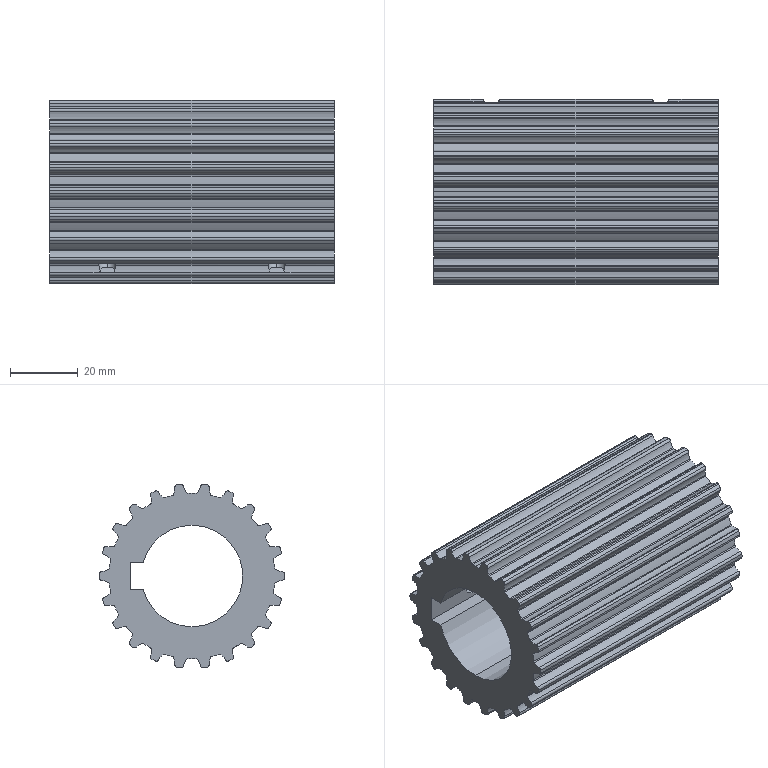Part | SolidWorks | features CirPattern 1, Cut 1, HoleWzd 1, ICE 1, WeldMemberFeat 1, WeldmentFeature 1 | 1 solid | 245 faces | box 84 x 54.65 x 54.249 mm | volume 111386 mm3 | cylinder 238 | plane 7 | commonest cylinder face diameters 0.8 x60 1.5 x60 10.6 x54 48.99 x29 54.65 x24 5 x8